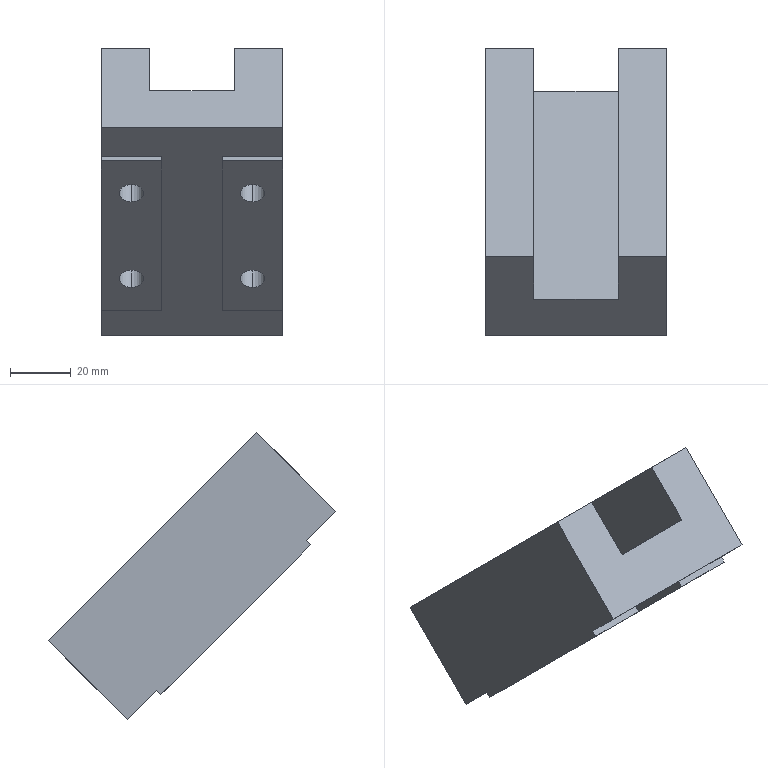Part | STEP file | X-Axis 28 Guide Rail Slider Block | 1 solid | 30 faces | box 60 x 95.035 x 95.035 mm | volume 165273 mm3 | plane 22 | cylinder 8 | commonest cylinder face diameters 8 x8
STEP:
#1=CARTESIAN_POINT('',(-793.,347.106,-240.707));
#2=VERTEX_POINT('',#1);
#3=CARTESIAN_POINT('',(-793.,352.762,-246.364));
#4=VERTEX_POINT('',#3);
#5=CARTESIAN_POINT('',(-793.,349.934,-243.536));
#6=DIRECTION('',(0.,-0.7071,-0.7071));
#7=DIRECTION('',(0.,0.7071,-0.7071));
#8=AXIS2_PLACEMENT_3D('',#5,#6,#7);
#9=CIRCLE('',#8,4.);
#10=EDGE_CURVE('',#2,#4,#9,.T.);
#11=ORIENTED_EDGE('',*,*,#10,.F.);
#12=CARTESIAN_POINT('',(-793.,340.034,-247.778));
#13=VERTEX_POINT('',#12);
#14=CARTESIAN_POINT('',(-793.,340.034,-247.778));
#15=DIRECTION('',(0.,-0.7071,-0.7071));
#16=VECTOR('',#15,1000.);
#17=LINE('',#14,#16);
#18=EDGE_CURVE('',#2,#13,#17,.T.);
#19=ORIENTED_EDGE('',*,*,#18,.T.);
#20=CARTESIAN_POINT('',(-793.,345.691,-253.435));
#21=VERTEX_POINT('',#20);
#22=CARTESIAN_POINT('',(-793.,342.863,-250.607));
#23=DIRECTION('',(0.,-0.7071,-0.7071));
#24=DIRECTION('',(0.,0.7071,-0.7071));
#25=AXIS2_PLACEMENT_3D('',#22,#23,#24);
#26=CIRCLE('',#25,4.);
#27=EDGE_CURVE('',#13,#21,#26,.T.);
#28=ORIENTED_EDGE('',*,*,#27,.T.);
#29=CARTESIAN_POINT('',(-793.,345.691,-253.435));
#30=DIRECTION('',(0.,-0.7071,-0.7071));
#31=VECTOR('',#30,1000.);
#32=LINE('',#29,#31);
#33=EDGE_CURVE('',#4,#21,#32,.T.);
#34=ORIENTED_EDGE('',*,*,#33,.F.);
#35=EDGE_LOOP('',(#11,#19,#28,#34));
#36=FACE_OUTER_BOUND('',#35,.T.);
#37=CARTESIAN_POINT('',(-793.,342.863,-250.607));
#38=DIRECTION('',(0.,-0.7071,-0.7071));
#39=DIRECTION('',(0.,0.7071,-0.7071));
#40=AXIS2_PLACEMENT_3D('',#37,#38,#39);
#41=CYLINDRICAL_SURFACE('',#40,4.);
#42=ADVANCED_FACE('',(#36),#41,.F.);
#43=CARTESIAN_POINT('',(-793.,375.39,-268.992));
#44=VERTEX_POINT('',#43);
#45=CARTESIAN_POINT('',(-793.,381.047,-274.649));
#46=VERTEX_POINT('',#45);
#47=CARTESIAN_POINT('',(-793.,378.218,-271.82));
#48=DIRECTION('',(0.,-0.7071,-0.7071));
#49=DIRECTION('',(0.,0.7071,-0.7071));
#50=AXIS2_PLACEMENT_3D('',#47,#48,#49);
#51=CIRCLE('',#50,4.);
#52=EDGE_CURVE('',#44,#46,#51,.T.);
#53=ORIENTED_EDGE('',*,*,#52,.F.);
#54=CARTESIAN_POINT('',(-793.,368.319,-276.063));
#55=VERTEX_POINT('',#54);
#56=CARTESIAN_POINT('',(-793.,368.319,-276.063));
#57=DIRECTION('',(0.,-0.7071,-0.7071));
#58=VECTOR('',#57,1000.);
#59=LINE('',#56,#58);
#60=EDGE_CURVE('',#44,#55,#59,.T.);
#61=ORIENTED_EDGE('',*,*,#60,.T.);
#62=CARTESIAN_POINT('',(-793.,373.976,-281.72));
#63=VERTEX_POINT('',#62);
#64=CARTESIAN_POINT('',(-793.,371.147,-278.891));
#65=DIRECTION('',(0.,-0.7071,-0.7071));
#66=DIRECTION('',(0.,0.7071,-0.7071));
#67=AXIS2_PLACEMENT_3D('',#64,#65,#66);
#68=CIRCLE('',#67,4.);
#69=EDGE_CURVE('',#55,#63,#68,.T.);
#70=ORIENTED_EDGE('',*,*,#69,.T.);
#71=CARTESIAN_POINT('',(-793.,373.976,-281.72));
#72=DIRECTION('',(0.,-0.7071,-0.7071));
#73=VECTOR('',#72,1000.);
#74=LINE('',#71,#73);
#75=EDGE_CURVE('',#46,#63,#74,.T.);
#76=ORIENTED_EDGE('',*,*,#75,.F.);
#77=EDGE_LOOP('',(#53,#61,#70,#76));
#78=FACE_OUTER_BOUND('',#77,.T.);
#79=CARTESIAN_POINT('',(-793.,371.147,-278.891));
#80=DIRECTION('',(0.,-0.7071,-0.7071));
#81=DIRECTION('',(0.,0.7071,-0.7071));
#82=AXIS2_PLACEMENT_3D('',#79,#80,#81);
#83=CYLINDRICAL_SURFACE('',#82,4.);
#84=ADVANCED_FACE('',(#78),#83,.F.);
#85=CARTESIAN_POINT('',(-753.,375.39,-268.992));
#86=VERTEX_POINT('',#85);
#87=CARTESIAN_POINT('',(-753.,381.047,-274.649));
#88=VERTEX_POINT('',#87);
#89=CARTESIAN_POINT('',(-753.,378.218,-271.82));
#90=DIRECTION('',(0.,-0.7071,-0.7071));
#91=DIRECTION('',(0.,0.7071,-0.7071));
#92=AXIS2_PLACEMENT_3D('',#89,#90,#91);
#93=CIRCLE('',#92,4.);
#94=EDGE_CURVE('',#86,#88,#93,.T.);
#95=ORIENTED_EDGE('',*,*,#94,.F.);
#96=CARTESIAN_POINT('',(-753.,368.319,-276.063));
#97=VERTEX_POINT('',#96);
#98=CARTESIAN_POINT('',(-753.,368.319,-276.063));
#99=DIRECTION('',(0.,-0.7071,-0.7071));
#100=VECTOR('',#99,1000.);
#101=LINE('',#98,#100);
#102=EDGE_CURVE('',#86,#97,#101,.T.);
#103=ORIENTED_EDGE('',*,*,#102,.T.);
#104=CARTESIAN_POINT('',(-753.,373.976,-281.72));
#105=VERTEX_POINT('',#104);
#106=CARTESIAN_POINT('',(-753.,371.147,-278.891));
#107=DIRECTION('',(0.,-0.7071,-0.7071));
#108=DIRECTION('',(0.,0.7071,-0.7071));
#109=AXIS2_PLACEMENT_3D('',#106,#107,#108);
#110=CIRCLE('',#109,4.);
#111=EDGE_CURVE('',#97,#105,#110,.T.);
#112=ORIENTED_EDGE('',*,*,#111,.T.);
#113=CARTESIAN_POINT('',(-753.,373.976,-281.72));
#114=DIRECTION('',(0.,-0.7071,-0.7071));
#115=VECTOR('',#114,1000.);
#116=LINE('',#113,#115);
#117=EDGE_CURVE('',#88,#105,#116,.T.);
#118=ORIENTED_EDGE('',*,*,#117,.F.);
#119=EDGE_LOOP('',(#95,#103,#112,#118));
#120=FACE_OUTER_BOUND('',#119,.T.);
#121=CARTESIAN_POINT('',(-753.,371.147,-278.891));
#122=DIRECTION('',(0.,-0.7071,-0.7071));
#123=DIRECTION('',(0.,0.7071,-0.7071));
#124=AXIS2_PLACEMENT_3D('',#121,#122,#123);
#125=CYLINDRICAL_SURFACE('',#124,4.);
#126=ADVANCED_FACE('',(#120),#125,.F.);
#127=CARTESIAN_POINT('',(-753.,347.106,-240.707));
#128=VERTEX_POINT('',#127);
#129=CARTESIAN_POINT('',(-753.,352.762,-246.364));
#130=VERTEX_POINT('',#129);
#131=CARTESIAN_POINT('',(-753.,349.934,-243.536));
#132=DIRECTION('',(0.,-0.7071,-0.7071));
#133=DIRECTION('',(0.,0.7071,-0.7071));
#134=AXIS2_PLACEMENT_3D('',#131,#132,#133);
#135=CIRCLE('',#134,4.);
#136=EDGE_CURVE('',#128,#130,#135,.T.);
#137=ORIENTED_EDGE('',*,*,#136,.F.);
#138=CARTESIAN_POINT('',(-753.,340.034,-247.778));
#139=VERTEX_POINT('',#138);
#140=CARTESIAN_POINT('',(-753.,340.034,-247.778));
#141=DIRECTION('',(0.,-0.7071,-0.7071));
#142=VECTOR('',#141,1000.);
#143=LINE('',#140,#142);
#144=EDGE_CURVE('',#128,#139,#143,.T.);
#145=ORIENTED_EDGE('',*,*,#144,.T.);
#146=CARTESIAN_POINT('',(-753.,345.691,-253.435));
#147=VERTEX_POINT('',#146);
#148=CARTESIAN_POINT('',(-753.,342.863,-250.607));
#149=DIRECTION('',(0.,-0.7071,-0.7071));
#150=DIRECTION('',(0.,0.7071,-0.7071));
#151=AXIS2_PLACEMENT_3D('',#148,#149,#150);
#152=CIRCLE('',#151,4.);
#153=EDGE_CURVE('',#139,#147,#152,.T.);
#154=ORIENTED_EDGE('',*,*,#153,.T.);
#155=CARTESIAN_POINT('',(-753.,345.691,-253.435));
#156=DIRECTION('',(0.,-0.7071,-0.7071));
#157=VECTOR('',#156,1000.);
#158=LINE('',#155,#157);
#159=EDGE_CURVE('',#130,#147,#158,.T.);
#160=ORIENTED_EDGE('',*,*,#159,.F.);
#161=EDGE_LOOP('',(#137,#145,#154,#160));
#162=FACE_OUTER_BOUND('',#161,.T.);
#163=CARTESIAN_POINT('',(-753.,342.863,-250.607));
#164=DIRECTION('',(0.,-0.7071,-0.7071));
#165=DIRECTION('',(0.,0.7071,-0.7071));
#166=AXIS2_PLACEMENT_3D('',#163,#164,#165);
#167=CYLINDRICAL_SURFACE('',#166,4.);
#168=ADVANCED_FACE('',(#162),#167,.F.);
#169=CARTESIAN_POINT('',(-803.,381.754,-289.498));
#170=VERTEX_POINT('',#169);
#171=CARTESIAN_POINT('',(-803.,332.256,-240.));
#172=VERTEX_POINT('',#171);
#173=CARTESIAN_POINT('',(-803.,381.754,-289.498));
#174=DIRECTION('',(0.,-0.7071,0.7071));
#175=VECTOR('',#174,1000.);
#176=LINE('',#173,#175);
#177=EDGE_CURVE('',#170,#172,#176,.T.);
#178=ORIENTED_EDGE('',*,*,#177,.T.);
#179=CARTESIAN_POINT('',(-803.,333.67,-238.586));
#180=VERTEX_POINT('',#179);
#181=CARTESIAN_POINT('',(-803.,332.256,-240.));
#182=DIRECTION('',(0.,0.7071,0.7071));
#183=VECTOR('',#182,1000.);
#184=LINE('',#181,#183);
#185=EDGE_CURVE('',#172,#180,#184,.T.);
#186=ORIENTED_EDGE('',*,*,#185,.T.);
#187=CARTESIAN_POINT('',(-803.,323.983,-228.899));
#188=VERTEX_POINT('',#187);
#189=CARTESIAN_POINT('',(-803.,333.67,-238.586));
#190=DIRECTION('',(0.,-0.7071,0.7071));
#191=VECTOR('',#190,1000.);
#192=LINE('',#189,#191);
#193=EDGE_CURVE('',#180,#188,#192,.T.);
#194=ORIENTED_EDGE('',*,*,#193,.T.);
#195=CARTESIAN_POINT('',(-803.,350.146,-202.736));
#196=VERTEX_POINT('',#195);
#197=CARTESIAN_POINT('',(-803.,323.983,-228.899));
#198=DIRECTION('',(0.,0.7071,0.7071));
#199=VECTOR('',#198,1000.);
#200=LINE('',#197,#199);
#201=EDGE_CURVE('',#188,#196,#200,.T.);
#202=ORIENTED_EDGE('',*,*,#201,.T.);
#203=CARTESIAN_POINT('',(-803.,419.018,-271.608));
#204=VERTEX_POINT('',#203);
#205=CARTESIAN_POINT('',(-803.,350.146,-202.736));
#206=DIRECTION('',(0.,0.7071,-0.7071));
#207=VECTOR('',#206,1000.);
#208=LINE('',#205,#207);
#209=EDGE_CURVE('',#196,#204,#208,.T.);
#210=ORIENTED_EDGE('',*,*,#209,.T.);
#211=CARTESIAN_POINT('',(-803.,392.855,-297.771));
#212=VERTEX_POINT('',#211);
#213=CARTESIAN_POINT('',(-803.,419.018,-271.608));
#214=DIRECTION('',(0.,-0.7071,-0.7071));
#215=VECTOR('',#214,1000.);
#216=LINE('',#213,#215);
#217=EDGE_CURVE('',#204,#212,#216,.T.);
#218=ORIENTED_EDGE('',*,*,#217,.T.);
#219=CARTESIAN_POINT('',(-803.,383.168,-288.084));
#220=VERTEX_POINT('',#219);
#221=CARTESIAN_POINT('',(-803.,392.855,-297.771));
#222=DIRECTION('',(0.,-0.7071,0.7071));
#223=VECTOR('',#222,1000.);
#224=LINE('',#221,#223);
#225=EDGE_CURVE('',#212,#220,#224,.T.);
#226=ORIENTED_EDGE('',*,*,#225,.T.);
#227=CARTESIAN_POINT('',(-803.,383.168,-288.084));
#228=DIRECTION('',(0.,-0.7071,-0.7071));
#229=VECTOR('',#228,1000.);
#230=LINE('',#227,#229);
#231=EDGE_CURVE('',#220,#170,#230,.T.);
#232=ORIENTED_EDGE('',*,*,#231,.T.);
#233=EDGE_LOOP('',(#178,#186,#194,#202,#210,#218,#226,#232));
#234=FACE_OUTER_BOUND('',#233,.T.);
#235=CARTESIAN_POINT('',(-803.,350.146,-202.736));
#236=DIRECTION('',(-1.,0.,0.));
#237=DIRECTION('',(0.,0.,1.));
#238=AXIS2_PLACEMENT_3D('',#235,#236,#237);
#239=PLANE('',#238);
#240=ADVANCED_FACE('',(#234),#239,.T.);
#241=ORIENTED_EDGE('',*,*,#185,.F.);
#242=CARTESIAN_POINT('',(-783.,332.256,-240.));
#243=VERTEX_POINT('',#242);
#244=CARTESIAN_POINT('',(-803.,332.256,-240.));
#245=DIRECTION('',(-1.,0.,0.));
#246=VECTOR('',#245,1000.);
#247=LINE('',#244,#246);
#248=EDGE_CURVE('',#243,#172,#247,.T.);
#249=ORIENTED_EDGE('',*,*,#248,.F.);
#250=CARTESIAN_POINT('',(-783.,333.67,-238.586));
#251=VERTEX_POINT('',#250);
#252=CARTESIAN_POINT('',(-783.,332.256,-240.));
#253=DIRECTION('',(0.,-0.7071,-0.7071));
#254=VECTOR('',#253,1000.);
#255=LINE('',#252,#254);
#256=EDGE_CURVE('',#251,#243,#255,.T.);
#257=ORIENTED_EDGE('',*,*,#256,.F.);
#258=CARTESIAN_POINT('',(-803.,333.67,-238.586));
#259=DIRECTION('',(1.,0.,0.));
#260=VECTOR('',#259,1000.);
#261=LINE('',#258,#260);
#262=EDGE_CURVE('',#180,#251,#261,.T.);
#263=ORIENTED_EDGE('',*,*,#262,.F.);
#264=EDGE_LOOP('',(#241,#249,#257,#263));
#265=FACE_OUTER_BOUND('',#264,.T.);
#266=CARTESIAN_POINT('',(-803.,332.256,-240.));
#267=DIRECTION('',(0.,0.7071,-0.7071));
#268=DIRECTION('',(0.,0.7071,0.7071));
#269=AXIS2_PLACEMENT_3D('',#266,#267,#268);
#270=PLANE('',#269);
#271=ADVANCED_FACE('',(#265),#270,.F.);
#272=CARTESIAN_POINT('',(-783.,381.754,-289.498));
#273=VERTEX_POINT('',#272);
#274=CARTESIAN_POINT('',(-783.,46.128,46.128));
#275=DIRECTION('',(0.,0.7071,-0.7071));
#276=VECTOR('',#275,1000.);
#277=LINE('',#274,#276);
#278=EDGE_CURVE('',#243,#273,#277,.T.);
#279=ORIENTED_EDGE('',*,*,#278,.F.);
#280=ORIENTED_EDGE('',*,*,#248,.T.);
#281=ORIENTED_EDGE('',*,*,#177,.F.);
#282=CARTESIAN_POINT('',(0.,381.754,-289.498));
#283=DIRECTION('',(-1.,0.,0.));
#284=VECTOR('',#283,1000.);
#285=LINE('',#282,#284);
#286=EDGE_CURVE('',#273,#170,#285,.T.);
#287=ORIENTED_EDGE('',*,*,#286,.F.);
#288=EDGE_LOOP('',(#279,#280,#281,#287));
#289=FACE_OUTER_BOUND('',#288,.T.);
#290=CARTESIAN_POINT('',(-793.,342.863,-250.607));
#291=DIRECTION('',(0.,-0.7071,-0.7071));
#292=DIRECTION('',(0.,0.7071,-0.7071));
#293=AXIS2_PLACEMENT_3D('',#290,#291,#292);
#294=CIRCLE('',#293,4.);
#295=EDGE_CURVE('',#21,#13,#294,.T.);
#296=ORIENTED_EDGE('',*,*,#295,.F.);
#297=ORIENTED_EDGE('',*,*,#27,.F.);
#298=EDGE_LOOP('',(#296,#297));
#299=FACE_BOUND('',#298,.T.);
#300=CARTESIAN_POINT('',(-793.,371.147,-278.891));
#301=DIRECTION('',(0.,-0.7071,-0.7071));
#302=DIRECTION('',(0.,0.7071,-0.7071));
#303=AXIS2_PLACEMENT_3D('',#300,#301,#302);
#304=CIRCLE('',#303,4.);
#305=EDGE_CURVE('',#63,#55,#304,.T.);
#306=ORIENTED_EDGE('',*,*,#305,.F.);
#307=ORIENTED_EDGE('',*,*,#69,.F.);
#308=EDGE_LOOP('',(#306,#307));
#309=FACE_BOUND('',#308,.T.);
#310=CARTESIAN_POINT('',(0.,46.128,46.128));
#311=DIRECTION('',(0.,0.7071,0.7071));
#312=DIRECTION('',(0.,-0.7071,0.7071));
#313=AXIS2_PLACEMENT_3D('',#310,#311,#312);
#314=PLANE('',#313);
#315=ADVANCED_FACE('',(#289,#299,#309),#314,.F.);
#316=CARTESIAN_POINT('',(-783.,383.168,-288.084));
#317=VERTEX_POINT('',#316);
#318=CARTESIAN_POINT('',(-783.,381.754,-289.498));
#319=DIRECTION('',(0.,0.7071,0.7071));
#320=VECTOR('',#319,1000.);
#321=LINE('',#318,#320);
#322=EDGE_CURVE('',#273,#317,#321,.T.);
#323=ORIENTED_EDGE('',*,*,#322,.F.);
#324=ORIENTED_EDGE('',*,*,#286,.T.);
#325=ORIENTED_EDGE('',*,*,#231,.F.);
#326=CARTESIAN_POINT('',(-783.,383.168,-288.084));
#327=DIRECTION('',(-1.,0.,0.));
#328=VECTOR('',#327,1000.);
#329=LINE('',#326,#328);
#330=EDGE_CURVE('',#317,#220,#329,.T.);
#331=ORIENTED_EDGE('',*,*,#330,.F.);
#332=EDGE_LOOP('',(#323,#324,#325,#331));
#333=FACE_OUTER_BOUND('',#332,.T.);
#334=CARTESIAN_POINT('',(-783.,381.754,-289.498));
#335=DIRECTION('',(0.,-0.7071,0.7071));
#336=DIRECTION('',(0.,-0.7071,-0.7071));
#337=AXIS2_PLACEMENT_3D('',#334,#335,#336);
#338=PLANE('',#337);
#339=ADVANCED_FACE('',(#333),#338,.F.);
#340=ORIENTED_EDGE('',*,*,#193,.F.);
#341=ORIENTED_EDGE('',*,*,#262,.T.);
#342=CARTESIAN_POINT('',(-783.,47.542,47.542));
#343=DIRECTION('',(0.,0.7071,-0.7071));
#344=VECTOR('',#343,1000.);
#345=LINE('',#342,#344);
#346=EDGE_CURVE('',#251,#317,#345,.T.);
#347=ORIENTED_EDGE('',*,*,#346,.T.);
#348=ORIENTED_EDGE('',*,*,#330,.T.);
#349=ORIENTED_EDGE('',*,*,#225,.F.);
#350=CARTESIAN_POINT('',(-743.,392.855,-297.771));
#351=VERTEX_POINT('',#350);
#352=CARTESIAN_POINT('',(0.,392.855,-297.771));
#353=DIRECTION('',(1.,0.,0.));
#354=VECTOR('',#353,1000.);
#355=LINE('',#352,#354);
#356=EDGE_CURVE('',#212,#351,#355,.T.);
#357=ORIENTED_EDGE('',*,*,#356,.T.);
#358=CARTESIAN_POINT('',(-743.,383.168,-288.084));
#359=VERTEX_POINT('',#358);
#360=CARTESIAN_POINT('',(-743.,47.542,47.542));
#361=DIRECTION('',(0.,-0.7071,0.7071));
#362=VECTOR('',#361,1000.);
#363=LINE('',#360,#362);
#364=EDGE_CURVE('',#351,#359,#363,.T.);
#365=ORIENTED_EDGE('',*,*,#364,.T.);
#366=CARTESIAN_POINT('',(-763.,383.168,-288.084));
#367=VERTEX_POINT('',#366);
#368=CARTESIAN_POINT('',(0.,383.168,-288.084));
#369=DIRECTION('',(-1.,0.,0.));
#370=VECTOR('',#369,1000.);
#371=LINE('',#368,#370);
#372=EDGE_CURVE('',#359,#367,#371,.T.);
#373=ORIENTED_EDGE('',*,*,#372,.T.);
#374=CARTESIAN_POINT('',(-763.,333.67,-238.586));
#375=VERTEX_POINT('',#374);
#376=CARTESIAN_POINT('',(-763.,47.542,47.542));
#377=DIRECTION('',(0.,-0.7071,0.7071));
#378=VECTOR('',#377,1000.);
#379=LINE('',#376,#378);
#380=EDGE_CURVE('',#367,#375,#379,.T.);
#381=ORIENTED_EDGE('',*,*,#380,.T.);
#382=CARTESIAN_POINT('',(-743.,333.67,-238.586));
#383=VERTEX_POINT('',#382);
#384=CARTESIAN_POINT('',(0.,333.67,-238.586));
#385=DIRECTION('',(1.,0.,0.));
#386=VECTOR('',#385,1000.);
#387=LINE('',#384,#386);
#388=EDGE_CURVE('',#375,#383,#387,.T.);
#389=ORIENTED_EDGE('',*,*,#388,.T.);
#390=CARTESIAN_POINT('',(-743.,323.983,-228.899));
#391=VERTEX_POINT('',#390);
#392=CARTESIAN_POINT('',(-743.,47.542,47.542));
#393=DIRECTION('',(0.,-0.7071,0.7071));
#394=VECTOR('',#393,1000.);
#395=LINE('',#392,#394);
#396=EDGE_CURVE('',#383,#391,#395,.T.);
#397=ORIENTED_EDGE('',*,*,#396,.T.);
#398=CARTESIAN_POINT('',(0.,323.983,-228.899));
#399=DIRECTION('',(-1.,0.,0.));
#400=VECTOR('',#399,1000.);
#401=LINE('',#398,#400);
#402=EDGE_CURVE('',#391,#188,#401,.T.);
#403=ORIENTED_EDGE('',*,*,#402,.T.);
#404=EDGE_LOOP('',(#340,#341,#347,#348,#349,#357,#365,#373,#381,#389,#397,#403));
#405=FACE_OUTER_BOUND('',#404,.T.);
#406=CARTESIAN_POINT('',(0.,47.542,47.542));
#407=DIRECTION('',(0.,-0.7071,-0.7071));
#408=DIRECTION('',(0.,0.7071,-0.7071));
#409=AXIS2_PLACEMENT_3D('',#406,#407,#408);
#410=PLANE('',#409);
#411=ADVANCED_FACE('',(#405),#410,.T.);
#412=ORIENTED_EDGE('',*,*,#217,.F.);
#413=CARTESIAN_POINT('',(-787.,419.018,-271.608));
#414=VERTEX_POINT('',#413);
#415=CARTESIAN_POINT('',(-803.,419.018,-271.608));
#416=DIRECTION('',(1.,0.,0.));
#417=VECTOR('',#416,1000.);
#418=LINE('',#415,#417);
#419=EDGE_CURVE('',#204,#414,#418,.T.);
#420=ORIENTED_EDGE('',*,*,#419,.T.);
#421=CARTESIAN_POINT('',(-787.,404.876,-285.75));
#422=VERTEX_POINT('',#421);
#423=CARTESIAN_POINT('',(-787.,419.018,-271.608));
#424=DIRECTION('',(0.,-0.7071,-0.7071));
#425=VECTOR('',#424,1000.);
#426=LINE('',#423,#425);
#427=EDGE_CURVE('',#414,#422,#426,.T.);
#428=ORIENTED_EDGE('',*,*,#427,.T.);
#429=CARTESIAN_POINT('',(-759.,404.876,-285.75));
#430=VERTEX_POINT('',#429);
#431=CARTESIAN_POINT('',(-803.,404.876,-285.75));
#432=DIRECTION('',(1.,0.,0.));
#433=VECTOR('',#432,1000.);
#434=LINE('',#431,#433);
#435=EDGE_CURVE('',#422,#430,#434,.T.);
#436=ORIENTED_EDGE('',*,*,#435,.T.);
#437=CARTESIAN_POINT('',(-759.,419.018,-271.608));
#438=VERTEX_POINT('',#437);
#439=CARTESIAN_POINT('',(-759.,419.018,-271.608));
#440=DIRECTION('',(0.,0.7071,0.7071));
#441=VECTOR('',#440,1000.);
#442=LINE('',#439,#441);
#443=EDGE_CURVE('',#430,#438,#442,.T.);
#444=ORIENTED_EDGE('',*,*,#443,.T.);
#445=CARTESIAN_POINT('',(-743.,419.018,-271.608));
#446=VERTEX_POINT('',#445);
#447=CARTESIAN_POINT('',(-803.,419.018,-271.608));
#448=DIRECTION('',(1.,0.,0.));
#449=VECTOR('',#448,1000.);
#450=LINE('',#447,#449);
#451=EDGE_CURVE('',#438,#446,#450,.T.);
#452=ORIENTED_EDGE('',*,*,#451,.T.);
#453=CARTESIAN_POINT('',(-743.,419.018,-271.608));
#454=DIRECTION('',(0.,-0.7071,-0.7071));
#455=VECTOR('',#454,1000.);
#456=LINE('',#453,#455);
#457=EDGE_CURVE('',#446,#351,#456,.T.);
#458=ORIENTED_EDGE('',*,*,#457,.T.);
#459=ORIENTED_EDGE('',*,*,#356,.F.);
#460=EDGE_LOOP('',(#412,#420,#428,#436,#444,#452,#458,#459));
#461=FACE_OUTER_BOUND('',#460,.T.);
#462=CARTESIAN_POINT('',(-803.,419.018,-271.608));
#463=DIRECTION('',(0.,0.7071,-0.7071));
#464=DIRECTION('',(0.,0.7071,0.7071));
#465=AXIS2_PLACEMENT_3D('',#462,#463,#464);
#466=PLANE('',#465);
#467=ADVANCED_FACE('',(#461),#466,.T.);
#468=CARTESIAN_POINT('',(-787.,350.146,-202.736));
#469=VERTEX_POINT('',#468);
#470=CARTESIAN_POINT('',(-787.,73.705,73.705));
#471=DIRECTION('',(0.,-0.7071,0.7071));
#472=VECTOR('',#471,1000.);
#473=LINE('',#470,#472);
#474=EDGE_CURVE('',#414,#469,#473,.T.);
#475=ORIENTED_EDGE('',*,*,#474,.F.);
#476=ORIENTED_EDGE('',*,*,#419,.F.);
#477=ORIENTED_EDGE('',*,*,#209,.F.);
#478=CARTESIAN_POINT('',(0.,350.146,-202.736));
#479=DIRECTION('',(-1.,0.,0.));
#480=VECTOR('',#479,1000.);
#481=LINE('',#478,#480);
#482=EDGE_CURVE('',#469,#196,#481,.T.);
#483=ORIENTED_EDGE('',*,*,#482,.F.);
#484=EDGE_LOOP('',(#475,#476,#477,#483));
#485=FACE_OUTER_BOUND('',#484,.T.);
#486=CARTESIAN_POINT('',(0.,73.705,73.705));
#487=DIRECTION('',(0.,-0.7071,-0.7071));
#488=DIRECTION('',(0.,0.7071,-0.7071));
#489=AXIS2_PLACEMENT_3D('',#486,#487,#488);
#490=PLANE('',#489);
#491=ADVANCED_FACE('',(#485),#490,.F.);
#492=CARTESIAN_POINT('',(-759.,350.146,-202.736));
#493=VERTEX_POINT('',#492);
#494=CARTESIAN_POINT('',(-759.,336.004,-216.878));
#495=VERTEX_POINT('',#494);
#496=CARTESIAN_POINT('',(-759.,350.146,-202.736));
#497=DIRECTION('',(0.,-0.7071,-0.7071));
#498=VECTOR('',#497,1000.);
#499=LINE('',#496,#498);
#500=EDGE_CURVE('',#493,#495,#499,.T.);
#501=ORIENTED_EDGE('',*,*,#500,.T.);
#502=CARTESIAN_POINT('',(-787.,336.004,-216.878));
#503=VERTEX_POINT('',#502);
#504=CARTESIAN_POINT('',(-743.,336.004,-216.878));
#505=DIRECTION('',(-1.,0.,0.));
#506=VECTOR('',#505,1000.);
#507=LINE('',#504,#506);
#508=EDGE_CURVE('',#495,#503,#507,.T.);
#509=ORIENTED_EDGE('',*,*,#508,.T.);
#510=CARTESIAN_POINT('',(-787.,350.146,-202.736));
#511=DIRECTION('',(0.,0.7071,0.7071));
#512=VECTOR('',#511,1000.);
#513=LINE('',#510,#512);
#514=EDGE_CURVE('',#503,#469,#513,.T.);
#515=ORIENTED_EDGE('',*,*,#514,.T.);
#516=ORIENTED_EDGE('',*,*,#482,.T.);
#517=ORIENTED_EDGE('',*,*,#201,.F.);
#518=ORIENTED_EDGE('',*,*,#402,.F.);
#519=CARTESIAN_POINT('',(-743.,350.146,-202.736));
#520=VERTEX_POINT('',#519);
#521=CARTESIAN_POINT('',(-743.,350.146,-202.736));
#522=DIRECTION('',(0.,0.7071,0.7071));
#523=VECTOR('',#522,1000.);
#524=LINE('',#521,#523);
#525=EDGE_CURVE('',#391,#520,#524,.T.);
#526=ORIENTED_EDGE('',*,*,#525,.T.);
#527=CARTESIAN_POINT('',(-743.,350.146,-202.736));
#528=DIRECTION('',(-1.,0.,0.));
#529=VECTOR('',#528,1000.);
#530=LINE('',#527,#529);
#531=EDGE_CURVE('',#520,#493,#530,.T.);
#532=ORIENTED_EDGE('',*,*,#531,.T.);
#533=EDGE_LOOP('',(#501,#509,#515,#516,#517,#518,#526,#532));
#534=FACE_OUTER_BOUND('',#533,.T.);
#535=CARTESIAN_POINT('',(-743.,350.146,-202.736));
#536=DIRECTION('',(0.,-0.7071,0.7071));
#537=DIRECTION('',(0.,-0.7071,-0.7071));
#538=AXIS2_PLACEMENT_3D('',#535,#536,#537);
#539=PLANE('',#538);
#540=ADVANCED_FACE('',(#534),#539,.T.);
#541=ORIENTED_EDGE('',*,*,#256,.T.);
#542=ORIENTED_EDGE('',*,*,#278,.T.);
#543=ORIENTED_EDGE('',*,*,#322,.T.);
#544=ORIENTED_EDGE('',*,*,#346,.F.);
#545=EDGE_LOOP('',(#541,#542,#543,#544));
#546=FACE_OUTER_BOUND('',#545,.T.);
#547=CARTESIAN_POINT('',(-783.,332.256,-240.));
#548=DIRECTION('',(-1.,0.,0.));
#549=DIRECTION('',(0.,0.,1.));
#550=AXIS2_PLACEMENT_3D('',#547,#548,#549);
#551=PLANE('',#550);
#552=ADVANCED_FACE('',(#546),#551,.F.);
#553=ORIENTED_EDGE('',*,*,#18,.F.);
#554=CARTESIAN_POINT('',(-793.,349.934,-243.536));
#555=DIRECTION('',(0.,-0.7071,-0.7071));
#556=DIRECTION('',(0.,0.7071,-0.7071));
#557=AXIS2_PLACEMENT_3D('',#554,#555,#556);
#558=CIRCLE('',#557,4.);
#559=EDGE_CURVE('',#4,#2,#558,.T.);
#560=ORIENTED_EDGE('',*,*,#559,.F.);
#561=ORIENTED_EDGE('',*,*,#33,.T.);
#562=ORIENTED_EDGE('',*,*,#295,.T.);
#563=EDGE_LOOP('',(#553,#560,#561,#562));
#564=FACE_OUTER_BOUND('',#563,.T.);
#565=CARTESIAN_POINT('',(-793.,342.863,-250.607));
#566=DIRECTION('',(0.,-0.7071,-0.7071));
#567=DIRECTION('',(0.,0.7071,-0.7071));
#568=AXIS2_PLACEMENT_3D('',#565,#566,#567);
#569=CYLINDRICAL_SURFACE('',#568,4.);
#570=ADVANCED_FACE('',(#564),#569,.F.);
#571=ORIENTED_EDGE('',*,*,#60,.F.);
#572=CARTESIAN_POINT('',(-793.,378.218,-271.82));
#573=DIRECTION('',(0.,-0.7071,-0.7071));
#574=DIRECTION('',(0.,0.7071,-0.7071));
#575=AXIS2_PLACEMENT_3D('',#572,#573,#574);
#576=CIRCLE('',#575,4.);
#577=EDGE_CURVE('',#46,#44,#576,.T.);
#578=ORIENTED_EDGE('',*,*,#577,.F.);
#579=ORIENTED_EDGE('',*,*,#75,.T.);
#580=ORIENTED_EDGE('',*,*,#305,.T.);
#581=EDGE_LOOP('',(#571,#578,#579,#580));
#582=FACE_OUTER_BOUND('',#581,.T.);
#583=CARTESIAN_POINT('',(-793.,371.147,-278.891));
#584=DIRECTION('',(0.,-0.7071,-0.7071));
#585=DIRECTION('',(0.,0.7071,-0.7071));
#586=AXIS2_PLACEMENT_3D('',#583,#584,#585);
#587=CYLINDRICAL_SURFACE('',#586,4.);
#588=ADVANCED_FACE('',(#582),#587,.F.);
#589=CARTESIAN_POINT('',(-743.,332.256,-240.));
#590=VERTEX_POINT('',#589);
#591=CARTESIAN_POINT('',(-743.,381.754,-289.498));
#592=VERTEX_POINT('',#591);
#593=CARTESIAN_POINT('',(-743.,332.256,-240.));
#594=DIRECTION('',(0.,0.7071,-0.7071));
#595=VECTOR('',#594,1000.);
#596=LINE('',#593,#595);
#597=EDGE_CURVE('',#590,#592,#596,.T.);
#598=ORIENTED_EDGE('',*,*,#597,.T.);
#599=CARTESIAN_POINT('',(-743.,381.754,-289.498));
#600=DIRECTION('',(0.,0.7071,0.7071));
#601=VECTOR('',#600,1000.);
#602=LINE('',#599,#601);
#603=EDGE_CURVE('',#592,#359,#602,.T.);
#604=ORIENTED_EDGE('',*,*,#603,.T.);
#605=ORIENTED_EDGE('',*,*,#364,.F.);
#606=ORIENTED_EDGE('',*,*,#457,.F.);
#607=CARTESIAN_POINT('',(-743.,419.018,-271.608));
#608=DIRECTION('',(0.,-0.7071,0.7071));
#609=VECTOR('',#608,1000.);
#610=LINE('',#607,#609);
#611=EDGE_CURVE('',#446,#520,#610,.T.);
#612=ORIENTED_EDGE('',*,*,#611,.T.);
#613=ORIENTED_EDGE('',*,*,#525,.F.);
#614=ORIENTED_EDGE('',*,*,#396,.F.);
#615=CARTESIAN_POINT('',(-743.,333.67,-238.586));
#616=DIRECTION('',(0.,-0.7071,-0.7071));
#617=VECTOR('',#616,1000.);
#618=LINE('',#615,#617);
#619=EDGE_CURVE('',#383,#590,#618,.T.);
#620=ORIENTED_EDGE('',*,*,#619,.T.);
#621=EDGE_LOOP('',(#598,#604,#605,#606,#612,#613,#614,#620));
#622=FACE_OUTER_BOUND('',#621,.T.);
#623=CARTESIAN_POINT('',(-743.,419.018,-271.608));
#624=DIRECTION('',(1.,0.,0.));
#625=DIRECTION('',(0.,0.,-1.));
#626=AXIS2_PLACEMENT_3D('',#623,#624,#625);
#627=PLANE('',#626);
#628=ADVANCED_FACE('',(#622),#627,.T.);
#629=CARTESIAN_POINT('',(-763.,332.256,-240.));
#630=VERTEX_POINT('',#629);
#631=CARTESIAN_POINT('',(-763.,332.256,-240.));
#632=DIRECTION('',(0.,0.7071,0.7071));
#633=VECTOR('',#632,1000.);
#634=LINE('',#631,#633);
#635=EDGE_CURVE('',#630,#375,#634,.T.);
#636=ORIENTED_EDGE('',*,*,#635,.F.);
#637=CARTESIAN_POINT('',(-763.,332.256,-240.));
#638=DIRECTION('',(-1.,0.,0.));
#639=VECTOR('',#638,1000.);
#640=LINE('',#637,#639);
#641=EDGE_CURVE('',#590,#630,#640,.T.);
#642=ORIENTED_EDGE('',*,*,#641,.F.);
#643=ORIENTED_EDGE('',*,*,#619,.F.);
#644=ORIENTED_EDGE('',*,*,#388,.F.);
#645=EDGE_LOOP('',(#636,#642,#643,#644));
#646=FACE_OUTER_BOUND('',#645,.T.);
#647=CARTESIAN_POINT('',(-763.,332.256,-240.));
#648=DIRECTION('',(0.,0.7071,-0.7071));
#649=DIRECTION('',(0.,0.7071,0.7071));
#650=AXIS2_PLACEMENT_3D('',#647,#648,#649);
#651=PLANE('',#650);
#652=ADVANCED_FACE('',(#646),#651,.F.);
#653=CARTESIAN_POINT('',(-763.,381.754,-289.498));
#654=VERTEX_POINT('',#653);
#655=CARTESIAN_POINT('',(-763.,381.754,-289.498));
#656=DIRECTION('',(0.,0.7071,0.7071));
#657=VECTOR('',#656,1000.);
#658=LINE('',#655,#657);
#659=EDGE_CURVE('',#654,#367,#658,.T.);
#660=ORIENTED_EDGE('',*,*,#659,.F.);
#661=CARTESIAN_POINT('',(-763.,332.256,-240.));
#662=DIRECTION('',(0.,0.7071,-0.7071));
#663=VECTOR('',#662,1000.);
#664=LINE('',#661,#663);
#665=EDGE_CURVE('',#630,#654,#664,.T.);
#666=ORIENTED_EDGE('',*,*,#665,.F.);
#667=ORIENTED_EDGE('',*,*,#635,.T.);
#668=ORIENTED_EDGE('',*,*,#380,.F.);
#669=EDGE_LOOP('',(#660,#666,#667,#668));
#670=FACE_OUTER_BOUND('',#669,.T.);
#671=CARTESIAN_POINT('',(-763.,381.754,-289.498));
#672=DIRECTION('',(1.,0.,0.));
#673=DIRECTION('',(0.,1.,0.));
#674=AXIS2_PLACEMENT_3D('',#671,#672,#673);
#675=PLANE('',#674);
#676=ADVANCED_FACE('',(#670),#675,.F.);
#677=ORIENTED_EDGE('',*,*,#603,.F.);
#678=CARTESIAN_POINT('',(-743.,381.754,-289.498));
#679=DIRECTION('',(1.,0.,0.));
#680=VECTOR('',#679,1000.);
#681=LINE('',#678,#680);
#682=EDGE_CURVE('',#654,#592,#681,.T.);
#683=ORIENTED_EDGE('',*,*,#682,.F.);
#684=ORIENTED_EDGE('',*,*,#659,.T.);
#685=ORIENTED_EDGE('',*,*,#372,.F.);
#686=EDGE_LOOP('',(#677,#683,#684,#685));
#687=FACE_OUTER_BOUND('',#686,.T.);
#688=CARTESIAN_POINT('',(-743.,381.754,-289.498));
#689=DIRECTION('',(0.,-0.7071,0.7071));
#690=DIRECTION('',(0.,-0.7071,-0.7071));
#691=AXIS2_PLACEMENT_3D('',#688,#689,#690);
#692=PLANE('',#691);
#693=ADVANCED_FACE('',(#687),#692,.F.);
#694=CARTESIAN_POINT('',(-759.,73.705,73.705));
#695=DIRECTION('',(0.,0.7071,-0.7071));
#696=VECTOR('',#695,1000.);
#697=LINE('',#694,#696);
#698=EDGE_CURVE('',#493,#438,#697,.T.);
#699=ORIENTED_EDGE('',*,*,#698,.F.);
#700=ORIENTED_EDGE('',*,*,#531,.F.);
#701=ORIENTED_EDGE('',*,*,#611,.F.);
#702=ORIENTED_EDGE('',*,*,#451,.F.);
#703=EDGE_LOOP('',(#699,#700,#701,#702));
#704=FACE_OUTER_BOUND('',#703,.T.);
#705=CARTESIAN_POINT('',(0.,73.705,73.705));
#706=DIRECTION('',(0.,-0.7071,-0.7071));
#707=DIRECTION('',(0.,0.7071,-0.7071));
#708=AXIS2_PLACEMENT_3D('',#705,#706,#707);
#709=PLANE('',#708);
#710=ADVANCED_FACE('',(#704),#709,.F.);
#711=ORIENTED_EDGE('',*,*,#698,.T.);
#712=ORIENTED_EDGE('',*,*,#443,.F.);
#713=CARTESIAN_POINT('',(-759.,336.004,-216.878));
#714=DIRECTION('',(0.,0.7071,-0.7071));
#715=VECTOR('',#714,1000.);
#716=LINE('',#713,#715);
#717=EDGE_CURVE('',#495,#430,#716,.T.);
#718=ORIENTED_EDGE('',*,*,#717,.F.);
#719=ORIENTED_EDGE('',*,*,#500,.F.);
#720=EDGE_LOOP('',(#711,#712,#718,#719));
#721=FACE_OUTER_BOUND('',#720,.T.);
#722=CARTESIAN_POINT('',(-759.,341.307,-185.412));
#723=DIRECTION('',(1.,0.,0.));
#724=DIRECTION('',(0.,0.,-1.));
#725=AXIS2_PLACEMENT_3D('',#722,#723,#724);
#726=PLANE('',#725);
#727=ADVANCED_FACE('',(#721),#726,.F.);
#728=ORIENTED_EDGE('',*,*,#717,.T.);
#729=ORIENTED_EDGE('',*,*,#435,.F.);
#730=CARTESIAN_POINT('',(-787.,322.922,-203.796));
#731=DIRECTION('',(0.,0.7071,-0.7071));
#732=VECTOR('',#731,1000.);
#733=LINE('',#730,#732);
#734=EDGE_CURVE('',#503,#422,#733,.T.);
#735=ORIENTED_EDGE('',*,*,#734,.F.);
#736=ORIENTED_EDGE('',*,*,#508,.F.);
#737=EDGE_LOOP('',(#728,#729,#735,#736));
#738=FACE_OUTER_BOUND('',#737,.T.);
#739=CARTESIAN_POINT('',(-759.,322.922,-203.796));
#740=DIRECTION('',(0.,-0.7071,-0.7071));
#741=DIRECTION('',(0.,0.7071,-0.7071));
#742=AXIS2_PLACEMENT_3D('',#739,#740,#741);
#743=PLANE('',#742);
#744=ADVANCED_FACE('',(#738),#743,.F.);
#745=ORIENTED_EDGE('',*,*,#734,.T.);
#746=ORIENTED_EDGE('',*,*,#427,.F.);
#747=ORIENTED_EDGE('',*,*,#474,.T.);
#748=ORIENTED_EDGE('',*,*,#514,.F.);
#749=EDGE_LOOP('',(#745,#746,#747,#748));
#750=FACE_OUTER_BOUND('',#749,.T.);
#751=CARTESIAN_POINT('',(-787.,322.922,-203.796));
#752=DIRECTION('',(-1.,0.,0.));
#753=DIRECTION('',(0.,0.,1.));
#754=AXIS2_PLACEMENT_3D('',#751,#752,#753);
#755=PLANE('',#754);
#756=ADVANCED_FACE('',(#750),#755,.F.);
#757=ORIENTED_EDGE('',*,*,#559,.T.);
#758=ORIENTED_EDGE('',*,*,#10,.T.);
#759=EDGE_LOOP('',(#757,#758));
#760=FACE_OUTER_BOUND('',#759,.T.);
#761=CARTESIAN_POINT('',(-793.,349.934,-243.536));
#762=DIRECTION('',(0.,0.7071,0.7071));
#763=DIRECTION('',(0.,-0.7071,0.7071));
#764=AXIS2_PLACEMENT_3D('',#761,#762,#763);
#765=PLANE('',#764);
#766=ADVANCED_FACE('',(#760),#765,.F.);
#767=ORIENTED_EDGE('',*,*,#577,.T.);
#768=ORIENTED_EDGE('',*,*,#52,.T.);
#769=EDGE_LOOP('',(#767,#768));
#770=FACE_OUTER_BOUND('',#769,.T.);
#771=CARTESIAN_POINT('',(-793.,378.218,-271.82));
#772=DIRECTION('',(0.,0.7071,0.7071));
#773=DIRECTION('',(0.,-0.7071,0.7071));
#774=AXIS2_PLACEMENT_3D('',#771,#772,#773);
#775=PLANE('',#774);
#776=ADVANCED_FACE('',(#770),#775,.F.);
#777=ORIENTED_EDGE('',*,*,#665,.T.);
#778=ORIENTED_EDGE('',*,*,#682,.T.);
#779=ORIENTED_EDGE('',*,*,#597,.F.);
#780=ORIENTED_EDGE('',*,*,#641,.T.);
#781=EDGE_LOOP('',(#777,#778,#779,#780));
#782=FACE_OUTER_BOUND('',#781,.T.);
#783=CARTESIAN_POINT('',(-753.,371.147,-278.891));
#784=DIRECTION('',(0.,-0.7071,-0.7071));
#785=DIRECTION('',(0.,0.7071,-0.7071));
#786=AXIS2_PLACEMENT_3D('',#783,#784,#785);
#787=CIRCLE('',#786,4.);
#788=EDGE_CURVE('',#105,#97,#787,.T.);
#789=ORIENTED_EDGE('',*,*,#788,.F.);
#790=ORIENTED_EDGE('',*,*,#111,.F.);
#791=EDGE_LOOP('',(#789,#790));
#792=FACE_BOUND('',#791,.T.);
#793=CARTESIAN_POINT('',(-753.,342.863,-250.607));
#794=DIRECTION('',(0.,-0.7071,-0.7071));
#795=DIRECTION('',(0.,0.7071,-0.7071));
#796=AXIS2_PLACEMENT_3D('',#793,#794,#795);
#797=CIRCLE('',#796,4.);
#798=EDGE_CURVE('',#147,#139,#797,.T.);
#799=ORIENTED_EDGE('',*,*,#798,.F.);
#800=ORIENTED_EDGE('',*,*,#153,.F.);
#801=EDGE_LOOP('',(#799,#800));
#802=FACE_BOUND('',#801,.T.);
#803=CARTESIAN_POINT('',(0.,46.128,46.128));
#804=DIRECTION('',(0.,0.7071,0.7071));
#805=DIRECTION('',(0.,-0.7071,0.7071));
#806=AXIS2_PLACEMENT_3D('',#803,#804,#805);
#807=PLANE('',#806);
#808=ADVANCED_FACE('',(#782,#792,#802),#807,.F.);
#809=ORIENTED_EDGE('',*,*,#102,.F.);
#810=CARTESIAN_POINT('',(-753.,378.218,-271.82));
#811=DIRECTION('',(0.,-0.7071,-0.7071));
#812=DIRECTION('',(0.,0.7071,-0.7071));
#813=AXIS2_PLACEMENT_3D('',#810,#811,#812);
#814=CIRCLE('',#813,4.);
#815=EDGE_CURVE('',#88,#86,#814,.T.);
#816=ORIENTED_EDGE('',*,*,#815,.F.);
#817=ORIENTED_EDGE('',*,*,#117,.T.);
#818=ORIENTED_EDGE('',*,*,#788,.T.);
#819=EDGE_LOOP('',(#809,#816,#817,#818));
#820=FACE_OUTER_BOUND('',#819,.T.);
#821=CARTESIAN_POINT('',(-753.,371.147,-278.891));
#822=DIRECTION('',(0.,-0.7071,-0.7071));
#823=DIRECTION('',(0.,0.7071,-0.7071));
#824=AXIS2_PLACEMENT_3D('',#821,#822,#823);
#825=CYLINDRICAL_SURFACE('',#824,4.);
#826=ADVANCED_FACE('',(#820),#825,.F.);
#827=ORIENTED_EDGE('',*,*,#144,.F.);
#828=CARTESIAN_POINT('',(-753.,349.934,-243.536));
#829=DIRECTION('',(0.,-0.7071,-0.7071));
#830=DIRECTION('',(0.,0.7071,-0.7071));
#831=AXIS2_PLACEMENT_3D('',#828,#829,#830);
#832=CIRCLE('',#831,4.);
#833=EDGE_CURVE('',#130,#128,#832,.T.);
#834=ORIENTED_EDGE('',*,*,#833,.F.);
#835=ORIENTED_EDGE('',*,*,#159,.T.);
#836=ORIENTED_EDGE('',*,*,#798,.T.);
#837=EDGE_LOOP('',(#827,#834,#835,#836));
#838=FACE_OUTER_BOUND('',#837,.T.);
#839=CARTESIAN_POINT('',(-753.,342.863,-250.607));
#840=DIRECTION('',(0.,-0.7071,-0.7071));
#841=DIRECTION('',(0.,0.7071,-0.7071));
#842=AXIS2_PLACEMENT_3D('',#839,#840,#841);
#843=CYLINDRICAL_SURFACE('',#842,4.);
#844=ADVANCED_FACE('',(#838),#843,.F.);
#845=ORIENTED_EDGE('',*,*,#815,.T.);
#846=ORIENTED_EDGE('',*,*,#94,.T.);
#847=EDGE_LOOP('',(#845,#846));
#848=FACE_OUTER_BOUND('',#847,.T.);
#849=CARTESIAN_POINT('',(-753.,378.218,-271.82));
#850=DIRECTION('',(0.,0.7071,0.7071));
#851=DIRECTION('',(0.,-0.7071,0.7071));
#852=AXIS2_PLACEMENT_3D('',#849,#850,#851);
#853=PLANE('',#852);
#854=ADVANCED_FACE('',(#848),#853,.F.);
#855=ORIENTED_EDGE('',*,*,#833,.T.);
#856=ORIENTED_EDGE('',*,*,#136,.T.);
#857=EDGE_LOOP('',(#855,#856));
#858=FACE_OUTER_BOUND('',#857,.T.);
#859=CARTESIAN_POINT('',(-753.,349.934,-243.536));
#860=DIRECTION('',(0.,0.7071,0.7071));
#861=DIRECTION('',(0.,-0.7071,0.7071));
#862=AXIS2_PLACEMENT_3D('',#859,#860,#861);
#863=PLANE('',#862);
#864=ADVANCED_FACE('',(#858),#863,.F.);
#865=CLOSED_SHELL('',(#42,#84,#126,#168,#240,#271,#315,#339,#411,#467,#491,#540,#552,#570,#588,#628,#652,#676,#693,#710,#727,#744,#756,#766,#776,#808,#826,#844,#854,#864));
#866=MANIFOLD_SOLID_BREP('',#865);
#867=CARTESIAN_POINT('',(0.,0.,0.));
#868=DIRECTION('',(0.,0.,1.));
#869=DIRECTION('',(1.,0.,0.));
#870=AXIS2_PLACEMENT_3D('',#867,#868,#869);
#871=(LENGTH_UNIT()NAMED_UNIT(*)SI_UNIT(.MILLI.,.METRE.));
#872=UNCERTAINTY_MEASURE_WITH_UNIT(LENGTH_MEASURE(0.00001),#871,'','');
#873=(NAMED_UNIT(*)PLANE_ANGLE_UNIT()SI_UNIT($,.RADIAN.));
#874=(NAMED_UNIT(*)SI_UNIT($,.STERADIAN.)SOLID_ANGLE_UNIT());
#875=(GEOMETRIC_REPRESENTATION_CONTEXT(3)GLOBAL_UNCERTAINTY_ASSIGNED_CONTEXT((#872))GLOBAL_UNIT_ASSIGNED_CONTEXT((#871,#873,#874))REPRESENTATION_CONTEXT('',''));
#876=ADVANCED_BREP_SHAPE_REPRESENTATION('',(#866,#870),#875);